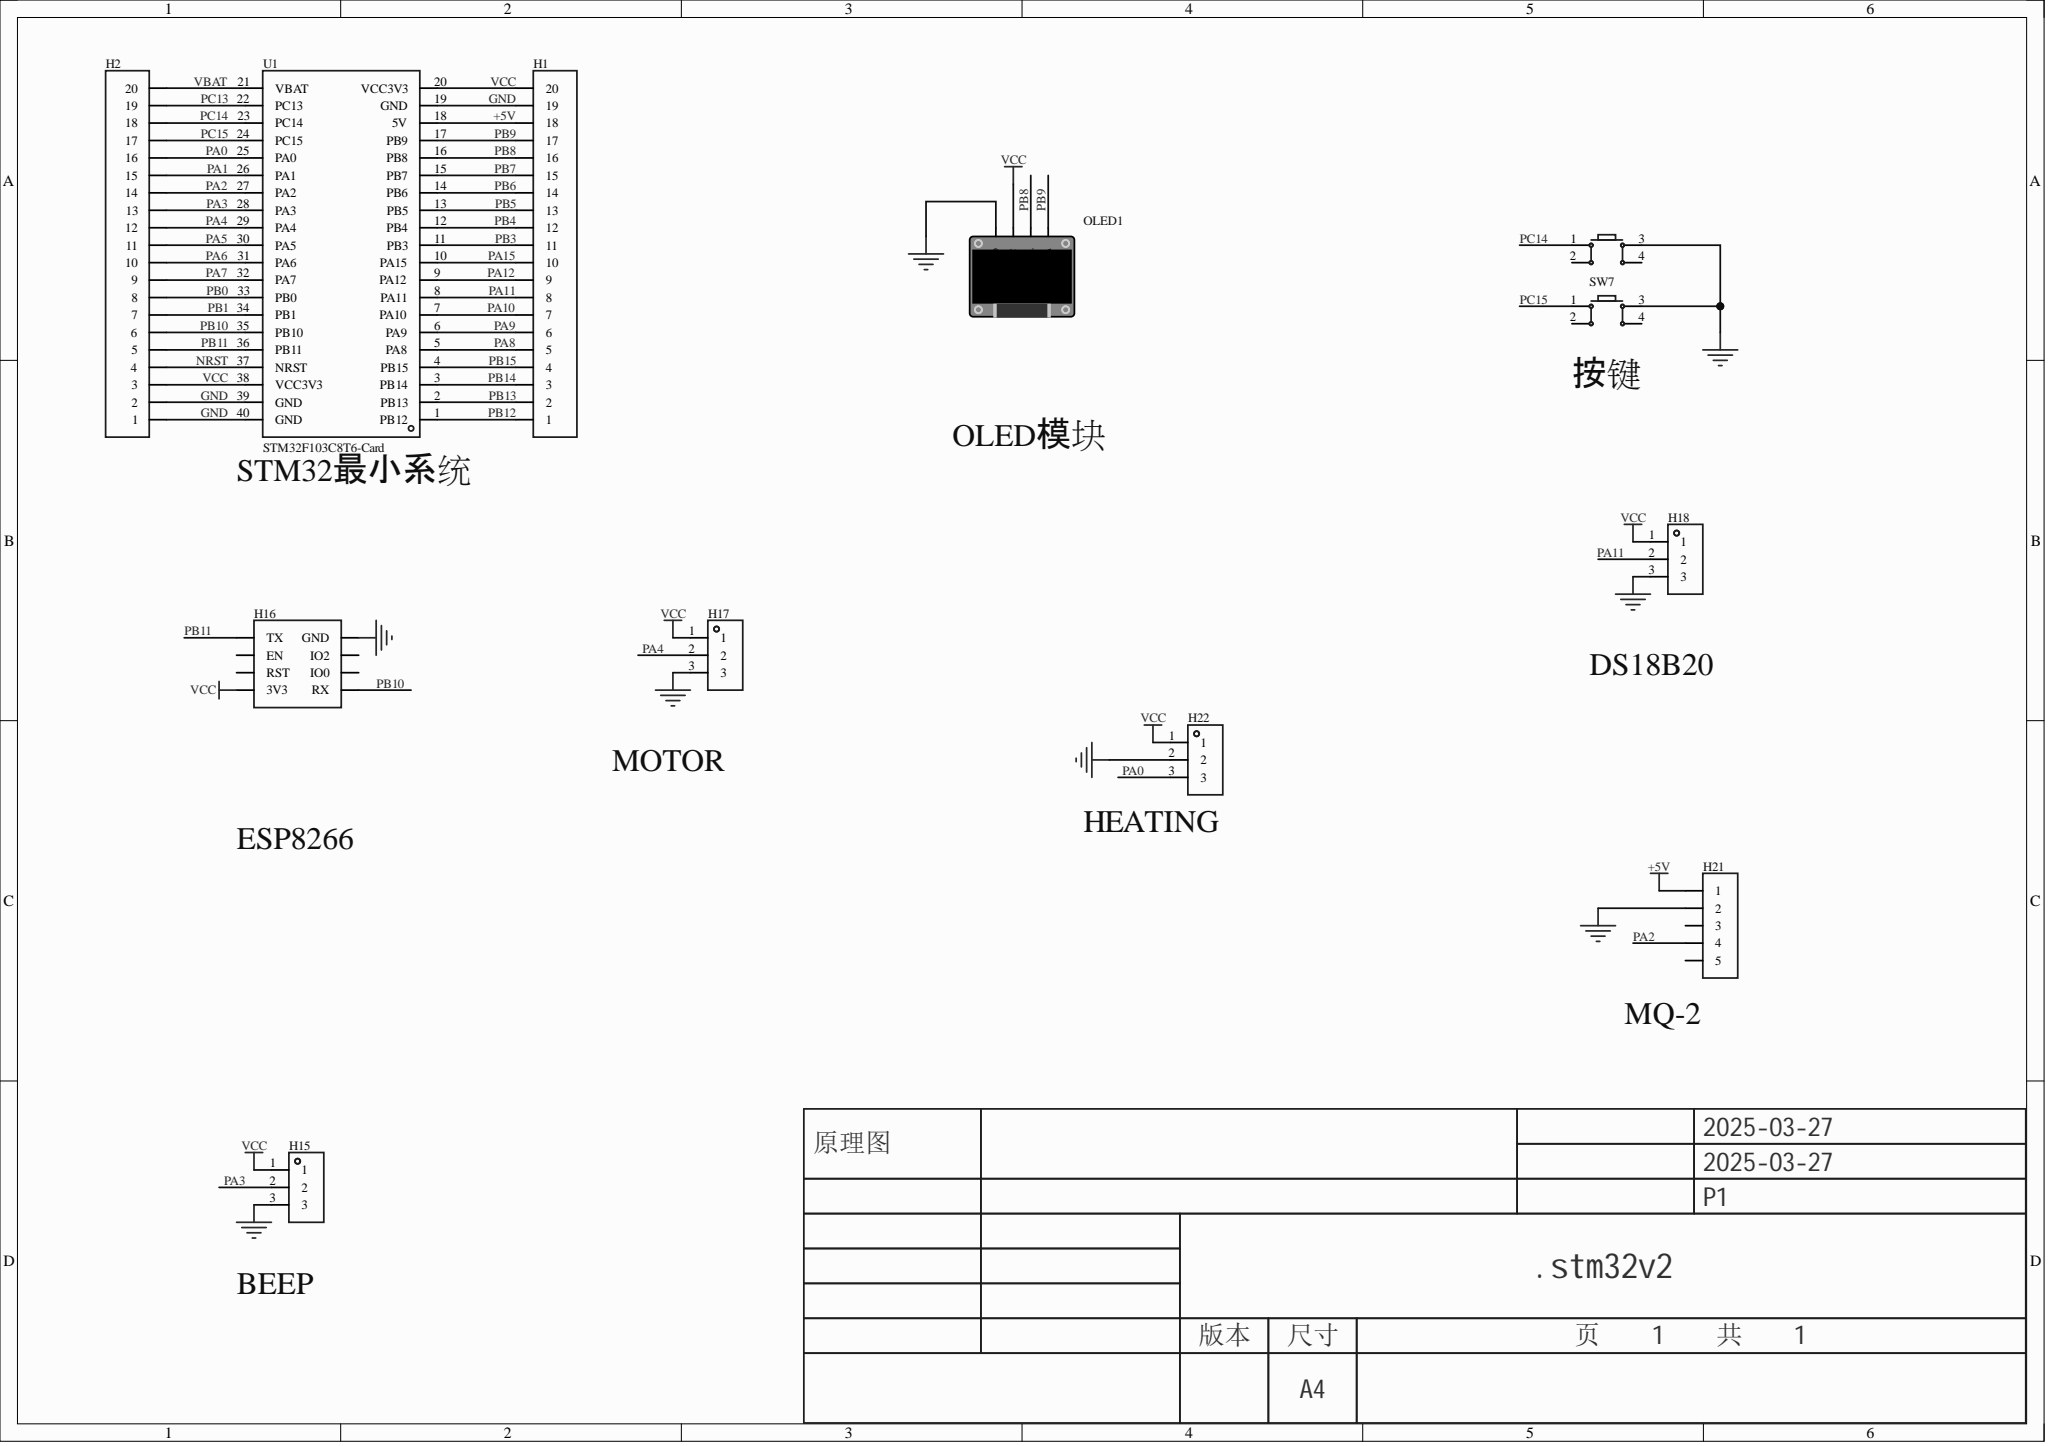Circuit board | Altium Designer | 12 parts | 37 nets
Bill of materials:
Comment,Description,Designator,Footprint,LibRef,Quantity
"","","H1, H2","HDR-TH_20P-P2.54-V-F","HDR-F_2.54_1x20P","2"
"","","H15, H17, H18, H22","HDR-TH_3P-P2.54-V-F","HDR-F_2.54_1x3P","4"
"","","H16","HDR-TH_8P-P2.54-V-F-R2-C4-S2.54-1","HDR-F_2.54_2x4","1"
"","","H21","HDR-TH_5P-P2.54-V-F","HDR-F_2.54_1x5P","1"
"","","OLED1","0.96OLED_4P","0.96OLED模块_4P","1"
"","","SW6, SW7","SW-TH_4P-L6.0-W6.0-P4.50-LS6.5","Key_TH_6x6x6","2"
"STM32F103C8T6-Card","","U1","CONN-TH_L53.3-W22.9_STM32F103C8T6-CARD","STM32F103C8T6-Card","1"
Netlist (Protel format):
[
H1
HDR-TH_20P-P2.54-V-F




]
[
H2
HDR-TH_20P-P2.54-V-F




]
[
H15
HDR-TH_3P-P2.54-V-F




]
[
H16
HDR-TH_8P-P2.54-V-F-R2-C4-S2.54-1




]
[
H17
HDR-TH_3P-P2.54-V-F




]
[
H18
HDR-TH_3P-P2.54-V-F




]
[
H21
HDR-TH_5P-P2.54-V-F




]
[
H22
HDR-TH_3P-P2.54-V-F




]
[
OLED1
0.96OLED_4P




]
[
SW6
SW-TH_4P-L6.0-W6.0-P4.50-LS6.5




]
[
SW7
SW-TH_4P-L6.0-W6.0-P4.50-LS6.5




]
[
U1
CONN-TH_L53.3-W22.9_STM32F103C8T6-CARD
STM32F103C8T6-Card



]
(
VCC
H1-20
H2-3
H15-1
H16-7
H17-1
H18-1
H22-1
OLED1-2
U1-20
U1-38
)
(
VBAT
H2-20
U1-21
)
(
PC15
H2-17
SW7-1
U1-24
)
(
PC14
H2-18
SW6-1
U1-23
)
(
PC13
H2-19
U1-22
)
(
PB15
H1-4
U1-4
)
(
PB14
H1-3
U1-3
)
(
PB13
H1-2
U1-2
)
(
PB12
H1-1
U1-1
)
(
PB11
H2-5
H16-1
U1-36
)
(
PB10
H2-6
H16-8
U1-35
)
(
PB9
H1-17
OLED1-4
U1-17
)
(
PB8
H1-16
OLED1-3
U1-16
)
(
PB7
H1-15
U1-15
)
(
PB6
H1-14
U1-14
)
(
PB5
H1-13
U1-13
)
(
PB4
H1-12
U1-12
)
(
PB3
H1-11
U1-11
)
(
PB1
H2-7
U1-34
)
(
PB0
H2-8
U1-33
)
(
PA15
H1-10
U1-10
)
(
PA12
H1-9
U1-9
)
(
PA11
H1-8
H18-2
U1-8
)
(
PA10
H1-7
U1-7
)
(
PA9
H1-6
U1-6
)
(
PA8
H1-5
U1-5
)
(
PA7
H2-9
U1-32
)
(
PA6
H2-10
U1-31
)
(
PA5
H2-11
U1-30
)
(
PA4
H2-12
H17-2
U1-29
)
(
PA3
H2-13
H15-2
U1-28
)
(
PA2
H2-14
H21-4
U1-27
)
(
PA1
H2-15
U1-26
)
(
PA0
H2-16
H22-3
U1-25
)
(
NRST
H2-4
U1-37
)
(
GND
H1-19
H2-1
H2-2
H15-3
H16-2
H17-3
H18-3
H21-2
H22-2
OLED1-1
SW6-3
SW7-3
U1-19
U1-39
U1-40
)
(
+5V
H1-18
H21-1
U1-18
)